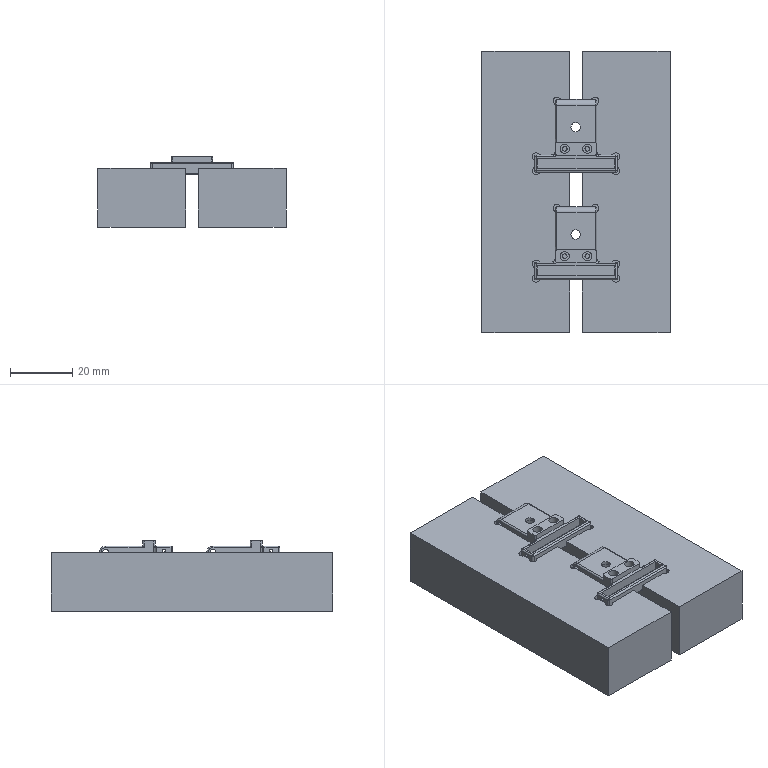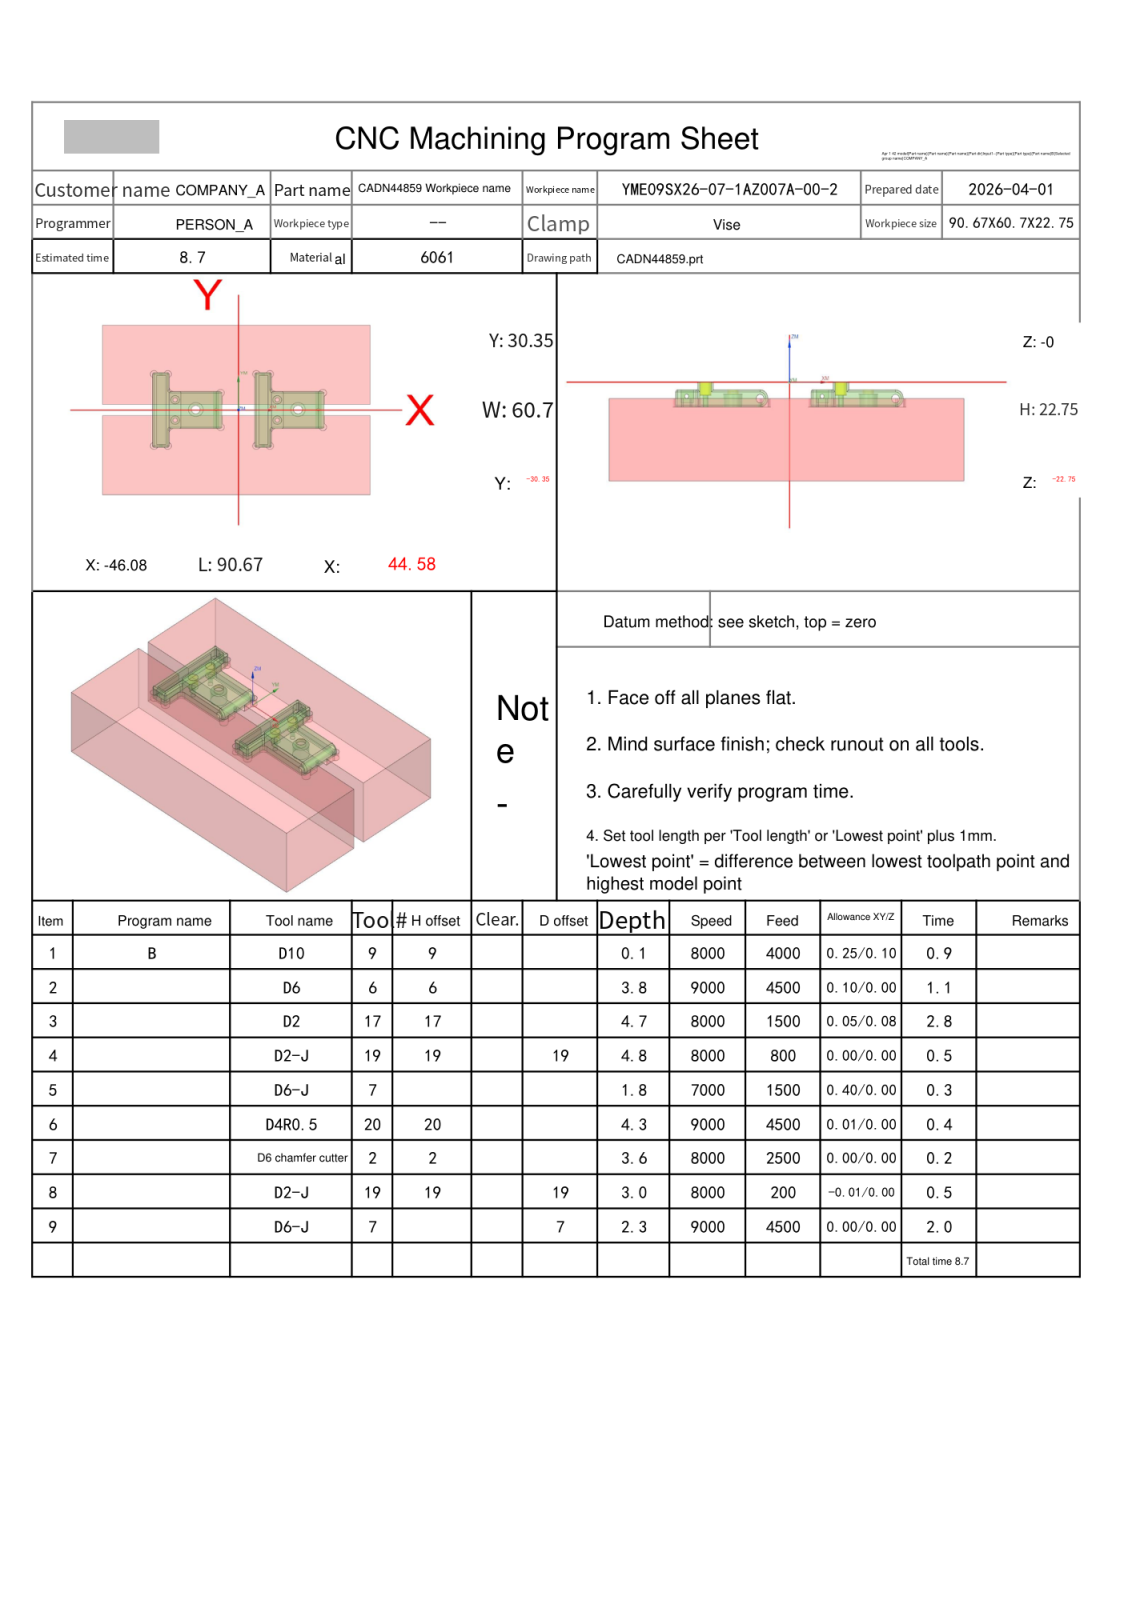NC program | NX | posted by the shop | part box 60.696 x 90.669 x 22.754 mm
Lines 1600 to 3624 of 6042, first 1509 of 2025 lines:
N3 T17 M06
(D2  D=2. R=0. H=17 ce=0.05 di=0.08)
G00 G90 G54 X-25.594 Y-2.915 M03 S8000
G43 H17 Z20.
M08
Z-.954
G01 Y11.298 Z-1.699 F1500.
X-26.646 Z-1.754
Y-11.298 Z-1.801
X-25.594 Z-1.803
Y11.298 Z-1.85
X-26.646 Z-1.852
Y-11.298 Z-1.899
X-25.594 Z-1.901
Y11.298 Z-1.948
X-26.646 Z-1.95
Y-11.298 Z-1.997
X-25.594 Z-1.999
Y11.298 Z-2.046
X-26.646 Z-2.048
Y-11.298 Z-2.095
X-25.594 Z-2.097
Y11.298 Z-2.144
X-26.646 Z-2.146
Y-11.298 Z-2.193
X-25.594 Z-2.195
Y11.298 Z-2.242
X-26.646 Z-2.244
Y-11.298 Z-2.291
X-25.594 Z-2.293
Y11.298 Z-2.34
X-26.646 Z-2.342
Y-11.298 Z-2.389
X-25.594 Z-2.391
Y11.298 Z-2.438
X-26.646 Z-2.44
Y-11.298 Z-2.487
X-25.594 Z-2.489
Y11.298 Z-2.536
X-26.646 Z-2.538
Y-11.298 Z-2.585
X-25.594 Z-2.587
Y11.298 Z-2.634
X-26.646 Z-2.636
Y-11.298 Z-2.683
X-25.594 Z-2.685
Y11.298 Z-2.732
X-26.646 Z-2.734
Y-11.298 Z-2.781
X-25.594 Z-2.783
Y11.298 Z-2.83
X-26.646 Z-2.832
Y-11.298 Z-2.879
X-25.594 Z-2.881
Y11.298 Z-2.928
X-26.646 Z-2.93
Y-11.298 Z-2.977
X-25.594 Z-2.979
Y11.298 Z-3.026
X-26.646 Z-3.028
Y-11.298 Z-3.075
X-25.594 Z-3.077
Y11.298 Z-3.124
X-26.646 Z-3.126
Y-11.298 Z-3.173
X-25.594 Z-3.175
Y11.298 Z-3.222
X-26.646 Z-3.224
Y-11.298 Z-3.271
X-25.594 Z-3.273
Y11.298 Z-3.32
X-26.646 Z-3.322
Y-11.298 Z-3.369
X-25.594 Z-3.371
Y11.298 Z-3.418
X-26.646 Z-3.42
Y-11.298 Z-3.467
X-25.594 Z-3.469
Y11.298 Z-3.516
X-26.646 Z-3.518
Y-11.298 Z-3.565
X-25.594 Z-3.567
Y11.298 Z-3.614
X-26.646 Z-3.616
Y-11.298 Z-3.663
X-25.594 Z-3.665
Y11.298 Z-3.712
X-26.646 Z-3.714
Y-11.298 Z-3.761
X-25.594 Z-3.763
Y11.298 Z-3.81
X-26.646 Z-3.812
Y-11.298 Z-3.859
X-25.594 Z-3.861
Y11.298 Z-3.908
X-26.646 Z-3.91
Y-11.298 Z-3.957
X-25.594 Z-3.959
Y11.298 Z-4.006
X-26.646 Z-4.008
Y-11.298 Z-4.055
X-25.594 Z-4.057
Y11.298 Z-4.104
X-26.646 Z-4.106
Y-11.298 Z-4.153
X-25.594 Z-4.155
Y11.298 Z-4.202
X-26.646 Z-4.204
Y-11.298 Z-4.251
X-25.594 Z-4.253
Y11.298 Z-4.3
X-26.646 Z-4.302
Y-11.298 Z-4.349
X-25.594 Z-4.351
Y11.298 Z-4.398
X-26.646 Z-4.4
Y-11.298 Z-4.447
X-25.594 Z-4.449
Y11.298 Z-4.496
X-26.646 Z-4.498
Y-11.298 Z-4.545
X-25.594 Z-4.547
Y11.298 Z-4.594
X-26.646 Z-4.596
Y-11.298 Z-4.643
X-25.594 Z-4.645
Y11.298 Z-4.692
X-26.646 Z-4.694
Y-11.298
X-25.594
Y11.298
X-26.646
Y10.898
Z-3.894
G00 Z20.
X9.006 Y-2.915
Z-.954
G01 Y11.298 Z-1.699
X7.954 Z-1.754
Y-11.298 Z-1.801
X9.006 Z-1.803
Y11.298 Z-1.85
X7.954 Z-1.852
Y-11.298 Z-1.899
X9.006 Z-1.901
Y11.298 Z-1.948
X7.954 Z-1.95
Y-11.298 Z-1.997
X9.006 Z-1.999
Y11.298 Z-2.046
X7.954 Z-2.048
Y-11.298 Z-2.095
X9.006 Z-2.097
Y11.298 Z-2.144
X7.954 Z-2.146
Y-11.298 Z-2.193
X9.006 Z-2.195
Y11.298 Z-2.242
X7.954 Z-2.244
Y-11.298 Z-2.291
X9.006 Z-2.293
Y11.298 Z-2.34
X7.954 Z-2.342
Y-11.298 Z-2.389
X9.006 Z-2.391
Y11.298 Z-2.438
X7.954 Z-2.44
Y-11.298 Z-2.487
X9.006 Z-2.489
Y11.298 Z-2.536
X7.954 Z-2.538
Y-11.298 Z-2.585
X9.006 Z-2.587
Y11.298 Z-2.634
X7.954 Z-2.636
Y-11.298 Z-2.683
X9.006 Z-2.685
Y11.298 Z-2.732
X7.954 Z-2.734
Y-11.298 Z-2.781
X9.006 Z-2.783
Y11.298 Z-2.83
X7.954 Z-2.832
Y-11.298 Z-2.879
X9.006 Z-2.881
Y11.298 Z-2.928
X7.954 Z-2.93
Y-11.298 Z-2.977
X9.006 Z-2.979
Y11.298 Z-3.026
X7.954 Z-3.028
Y-11.298 Z-3.075
X9.006 Z-3.077
Y11.298 Z-3.124
X7.954 Z-3.126
Y-11.298 Z-3.173
X9.006 Z-3.175
Y11.298 Z-3.222
X7.954 Z-3.224
Y-11.298 Z-3.271
X9.006 Z-3.273
Y11.298 Z-3.32
X7.954 Z-3.322
Y-11.298 Z-3.369
X9.006 Z-3.371
Y11.298 Z-3.418
X7.954 Z-3.42
Y-11.298 Z-3.467
X9.006 Z-3.469
Y11.298 Z-3.516
X7.954 Z-3.518
Y-11.298 Z-3.565
X9.006 Z-3.567
Y11.298 Z-3.614
X7.954 Z-3.616
Y-11.298 Z-3.663
X9.006 Z-3.665
Y11.298 Z-3.712
X7.954 Z-3.714
Y-11.298 Z-3.761
X9.006 Z-3.763
Y11.298 Z-3.81
X7.954 Z-3.812
Y-11.298 Z-3.859
X9.006 Z-3.861
Y11.298 Z-3.908
X7.954 Z-3.91
Y-11.298 Z-3.957
X9.006 Z-3.959
Y11.298 Z-4.006
X7.954 Z-4.008
Y-11.298 Z-4.055
X9.006 Z-4.057
Y11.298 Z-4.104
X7.954 Z-4.106
Y-11.298 Z-4.153
X9.006 Z-4.155
Y11.298 Z-4.202
X7.954 Z-4.204
Y-11.298 Z-4.251
X9.006 Z-4.253
Y11.298 Z-4.3
X7.954 Z-4.302
Y-11.298 Z-4.349
X9.006 Z-4.351
Y11.298 Z-4.398
X7.954 Z-4.4
Y-11.298 Z-4.447
X9.006 Z-4.449
Y11.298 Z-4.496
X7.954 Z-4.498
Y-11.298 Z-4.545
X9.006 Z-4.547
Y11.298 Z-4.594
X7.954 Z-4.596
Y-11.298 Z-4.643
X9.006 Z-4.645
Y11.298 Z-4.692
X7.954 Z-4.694
Y-11.298
X9.006
Y11.298
X7.954
Y10.898
Z-3.894
G00 Z20.
G00 G90 X13.59 Y3.809 M03 S8000
Z20.
Z.8
G01 X13.315 Y4.084 Z.78 F500.
X12.981 Z.762
X12.698 Y3.801 Z.741
Y3.471 Z.724
X12.981 Y3.184 Z.702
X13.315 Z.685
X13.598 Y3.467 Z.664
Y3.801 Z.646
X13.315 Y4.084 Z.625
X12.981 Z.608
X12.698 Y3.801 Z.587
Y3.471 Z.57
X12.981 Y3.184 Z.548
X13.315 Z.531
X13.598 Y3.467 Z.51
Y3.801 Z.492
X13.315 Y4.084 Z.471
X12.981 Z.454
X12.698 Y3.801 Z.433
Y3.471 Z.416
X12.981 Y3.184 Z.394
X13.315 Z.377
X13.598 Y3.467 Z.356
Y3.801 Z.338
X13.315 Y4.084 Z.317
X12.981 Z.3
X12.698 Y3.801 Z.279
Y3.471 Z.261
X12.981 Y3.184 Z.24
X13.315 Z.222
X13.598 Y3.467 Z.201
Y3.801 Z.184
X13.315 Y4.084 Z.163
X12.981 Z.145
X12.698 Y3.801 Z.124
Y3.471 Z.107
X12.981 Y3.184 Z.086
X13.315 Z.068
X13.598 Y3.467 Z.047
Y3.801 Z.03
X13.315 Y4.084 Z.009
X13.148 Z0.0
G03 X12.698 Y3.634 Z-.025 I0.0 J-.45
X12.802 Y3.346 Z-.035 I.45 J0.0
X13.148 Y3.184 Z-.049 I.346 J.288
X13.598 Y3.634 Z-.074 I0.0 J.45
X13.148 Y4.084 Z-.098 I-.45 J0.0
X12.698 Y3.634 Z-.123 I0.0 J-.45
X12.802 Y3.346 Z-.133 I.45 J0.0
X13.148 Y3.184 Z-.147 I.346 J.288
X13.598 Y3.634 Z-.172 I0.0 J.45
X13.148 Y4.084 Z-.196 I-.45 J0.0
X12.698 Y3.634 Z-.22 I0.0 J-.45
X12.802 Y3.346 Z-.231 I.45 J0.0
X13.148 Y3.184 Z-.245 I.346 J.288
X13.598 Y3.634 Z-.269 I0.0 J.45
X13.148 Y4.084 Z-.294 I-.45 J0.0
X12.698 Y3.634 Z-.318 I0.0 J-.45
X12.802 Y3.346 Z-.329 I.45 J0.0
X13.148 Y3.184 Z-.343 I.346 J.288
X13.598 Y3.634 Z-.367 I0.0 J.45
X13.148 Y4.084 Z-.392 I-.45 J0.0
X12.698 Y3.634 Z-.416 I0.0 J-.45
X12.802 Y3.346 Z-.427 I.45 J0.0
X13.148 Y3.184 Z-.441 I.346 J.288
X13.598 Y3.634 Z-.465 I0.0 J.45
X13.148 Y4.084 Z-.49 I-.45 J0.0
X12.698 Y3.634 Z-.514 I0.0 J-.45
X12.802 Y3.346 Z-.525 I.45 J0.0
X13.148 Y3.184 Z-.539 I.346 J.288
X13.598 Y3.634 Z-.563 I0.0 J.45
X13.148 Y4.084 Z-.588 I-.45 J0.0
X12.698 Y3.634 Z-.612 I0.0 J-.45
X12.802 Y3.346 Z-.623 I.45 J0.0
X13.148 Y3.184 Z-.637 I.346 J.288
X13.598 Y3.634 Z-.661 I0.0 J.45
X13.148 Y4.084 Z-.686 I-.45 J0.0
X12.698 Y3.634 Z-.71 I0.0 J-.45
X12.802 Y3.346 Z-.721 I.45 J0.0
X13.148 Y3.184 Z-.735 I.346 J.288
X13.598 Y3.634 Z-.759 I0.0 J.45
X13.148 Y4.084 Z-.784 I-.45 J0.0
X12.698 Y3.634 Z-.808 I0.0 J-.45
X12.802 Y3.346 Z-.819 I.45 J0.0
X13.148 Y3.184 Z-.833 I.346 J.288
X13.598 Y3.634 Z-.857 I0.0 J.45
X13.148 Y4.084 Z-.882 I-.45 J0.0
X12.698 Y3.634 Z-.906 I0.0 J-.45
X12.802 Y3.346 Z-.917 I.45 J0.0
X13.148 Y3.184 Z-.931 I.346 J.288
X13.598 Y3.634 Z-.955 I0.0 J.45
X13.148 Y4.084 Z-.98 I-.45 J0.0
X12.698 Y3.634 Z-1.004 I0.0 J-.45
X12.802 Y3.346 Z-1.015 I.45 J0.0
X13.148 Y3.184 Z-1.029 I.346 J.288
X13.598 Y3.634 Z-1.053 I0.0 J.45
X13.148 Y4.084 Z-1.078 I-.45 J0.0
X12.698 Y3.634 Z-1.102 I0.0 J-.45
X12.802 Y3.346 Z-1.113 I.45 J0.0
X13.148 Y3.184 Z-1.127 I.346 J.288
X13.598 Y3.634 Z-1.151 I0.0 J.45
X13.148 Y4.084 Z-1.176 I-.45 J0.0
X12.698 Y3.634 Z-1.2 I0.0 J-.45
X12.802 Y3.346 Z-1.211 I.45 J0.0
X13.148 Y3.184 Z-1.225 I.346 J.288
X13.598 Y3.634 Z-1.249 I0.0 J.45
X13.148 Y4.084 Z-1.274 I-.45 J0.0
X12.698 Y3.634 Z-1.298 I0.0 J-.45
X12.802 Y3.346 Z-1.309 I.45 J0.0
X13.148 Y3.184 Z-1.323 I.346 J.288
X13.598 Y3.634 Z-1.347 I0.0 J.45
X13.148 Y4.084 Z-1.372 I-.45 J0.0
X12.698 Y3.634 Z-1.396 I0.0 J-.45
X12.802 Y3.346 Z-1.407 I.45 J0.0
X13.148 Y3.184 Z-1.421 I.346 J.288
X13.598 Y3.634 Z-1.445 I0.0 J.45
X13.148 Y4.084 Z-1.47 I-.45 J0.0
X12.698 Y3.634 Z-1.494 I0.0 J-.45
X12.802 Y3.346 Z-1.505 I.45 J0.0
X13.148 Y3.184 Z-1.519 I.346 J.288
X13.598 Y3.634 Z-1.543 I0.0 J.45
X13.148 Y4.084 Z-1.568 I-.45 J0.0
X12.698 Y3.634 Z-1.592 I0.0 J-.45
X12.802 Y3.346 Z-1.603 I.45 J0.0
X13.148 Y3.184 Z-1.617 I.346 J.288
X13.598 Y3.634 Z-1.641 I0.0 J.45
X13.148 Y4.084 Z-1.666 I-.45 J0.0
X12.698 Y3.634 Z-1.69 I0.0 J-.45
X12.802 Y3.346 Z-1.701 I.45 J0.0
X13.148 Y3.184 Z-1.715 I.346 J.288
X13.598 Y3.634 Z-1.739 I0.0 J.45
X13.148 Y4.084 Z-1.764 I-.45 J0.0
X12.698 Y3.634 Z-1.788 I0.0 J-.45
X12.802 Y3.346 Z-1.799 I.45 J0.0
X13.148 Y3.184 Z-1.813 I.346 J.288
X13.598 Y3.634 Z-1.837 I0.0 J.45
X13.148 Y4.084 Z-1.862 I-.45 J0.0
X12.698 Y3.634 Z-1.886 I0.0 J-.45
X12.802 Y3.346 Z-1.897 I.45 J0.0
X13.148 Y3.184 Z-1.911 I.346 J.288
X13.598 Y3.634 Z-1.935 I0.0 J.45
X13.148 Y4.084 Z-1.96 I-.45 J0.0
X12.698 Y3.634 Z-1.984 I0.0 J-.45
X12.802 Y3.346 Z-1.995 I.45 J0.0
X13.148 Y3.184 Z-2.009 I.346 J.288
X13.598 Y3.634 Z-2.033 I0.0 J.45
X13.148 Y4.084 Z-2.058 I-.45 J0.0
X12.698 Y3.634 Z-2.082 I0.0 J-.45
X12.802 Y3.346 Z-2.093 I.45 J0.0
X13.148 Y3.184 Z-2.107 I.346 J.288
X13.598 Y3.634 Z-2.131 I0.0 J.45
X13.148 Y4.084 Z-2.156 I-.45 J0.0
X12.698 Y3.634 Z-2.18 I0.0 J-.45
X12.802 Y3.346 Z-2.191 I.45 J0.0
X13.148 Y3.184 Z-2.205 I.346 J.288
X13.598 Y3.634 Z-2.229 I0.0 J.45
X13.148 Y4.084 Z-2.254 I-.45 J0.0
X12.698 Y3.634 Z-2.278 I0.0 J-.45
X12.802 Y3.346 Z-2.289 I.45 J0.0
X13.148 Y3.184 Z-2.303 I.346 J.288
X13.598 Y3.634 Z-2.327 I0.0 J.45
X13.148 Y4.084 Z-2.352 I-.45 J0.0
X12.698 Y3.634 Z-2.376 I0.0 J-.45
X12.802 Y3.346 Z-2.387 I.45 J0.0
X13.148 Y3.184 Z-2.401 I.346 J.288
X13.598 Y3.634 Z-2.425 I0.0 J.45
X13.148 Y4.084 Z-2.45 I-.45 J0.0
X12.698 Y3.634 Z-2.474 I0.0 J-.45
X12.802 Y3.346 Z-2.485 I.45 J0.0
X13.148 Y3.184 Z-2.499 I.346 J.288
X13.598 Y3.634 Z-2.523 I0.0 J.45
X13.148 Y4.084 Z-2.548 I-.45 J0.0
X12.698 Y3.634 Z-2.572 I0.0 J-.45
X12.802 Y3.346 Z-2.583 I.45 J0.0
X13.148 Y3.184 Z-2.597 I.346 J.288
X13.598 Y3.634 Z-2.621 I0.0 J.45
X13.148 Y4.084 Z-2.646 I-.45 J0.0
X12.698 Y3.634 Z-2.67 I0.0 J-.45
X12.802 Y3.346 Z-2.681 I.45 J0.0
X13.148 Y3.184 Z-2.695 I.346 J.288
X13.598 Y3.634 Z-2.719 I0.0 J.45
X13.148 Y4.084 Z-2.744 I-.45 J0.0
X12.698 Y3.634 Z-2.768 I0.0 J-.45
X12.802 Y3.346 Z-2.779 I.45 J0.0
X13.148 Y3.184 Z-2.793 I.346 J.288
X13.598 Y3.634 Z-2.817 I0.0 J.45
X13.148 Y4.084 Z-2.842 I-.45 J0.0
X12.698 Y3.634 Z-2.866 I0.0 J-.45
X12.802 Y3.346 Z-2.877 I.45 J0.0
X13.148 Y3.184 Z-2.891 I.346 J.288
X13.598 Y3.634 Z-2.915 I0.0 J.45
X13.148 Y4.084 Z-2.94 I-.45 J0.0
X12.698 Y3.634 I0.0 J-.45
X13.148 Y3.184 I.45 J0.0
X13.598 Y3.634 I0.0 J.45
X13.148 Y4.084 I-.45 J0.0
X12.798 Y3.917 I0.0 J-.45
G01 Z-2.14
G00 Z20.
X12.698 Y-3.788
Z.8
G01 Y-3.801 Z.799
X12.981 Y-4.084 Z.778
X13.315 Z.761
X13.598 Y-3.801 Z.74
Y-3.467 Z.722
X13.315 Y-3.184 Z.701
X12.981 Z.684
X12.698 Y-3.467 Z.663
Y-3.801 Z.645
X12.981 Y-4.084 Z.624
X13.315 Z.607
X13.598 Y-3.801 Z.586
Y-3.467 Z.568
X13.315 Y-3.184 Z.547
X12.981 Z.53
X12.698 Y-3.467 Z.509
Y-3.801 Z.491
X12.981 Y-4.084 Z.471
X13.315 Z.453
X13.598 Y-3.801 Z.432
Y-3.467 Z.415
X13.315 Y-3.184 Z.394
X12.981 Z.376
X12.698 Y-3.467 Z.355
Y-3.801 Z.338
X12.981 Y-4.084 Z.317
X13.315 Z.299
X13.598 Y-3.801 Z.278
Y-3.467 Z.261
X13.315 Y-3.184 Z.24
X12.981 Z.222
X12.698 Y-3.467 Z.201
Y-3.801 Z.184
X12.981 Y-4.084 Z.163
X13.315 Z.145
X13.598 Y-3.801 Z.124
Y-3.467 Z.107
X13.315 Y-3.184 Z.086
X12.981 Z.068
X12.698 Y-3.467 Z.047
Y-3.801 Z.03
X12.981 Y-4.084 Z.009
X13.148 Z0.0
G03 X13.598 Y-3.634 Z-.025 I0.0 J.45
X13.148 Y-3.184 Z-.049 I-.45 J0.0
X12.698 Y-3.634 Z-.074 I0.0 J-.45
X13.148 Y-4.084 Z-.098 I.45 J0.0
X13.598 Y-3.634 Z-.123 I0.0 J.45
X13.148 Y-3.184 Z-.147 I-.45 J0.0
X12.698 Y-3.634 Z-.172 I0.0 J-.45
X13.148 Y-4.084 Z-.196 I.45 J0.0
X13.598 Y-3.634 Z-.22 I0.0 J.45
X13.148 Y-3.184 Z-.245 I-.45 J0.0
X12.698 Y-3.634 Z-.269 I0.0 J-.45
X13.148 Y-4.084 Z-.294 I.45 J0.0
X13.598 Y-3.634 Z-.318 I0.0 J.45
X13.148 Y-3.184 Z-.343 I-.45 J0.0
X12.698 Y-3.634 Z-.367 I0.0 J-.45
X13.148 Y-4.084 Z-.392 I.45 J0.0
X13.598 Y-3.634 Z-.416 I0.0 J.45
X13.148 Y-3.184 Z-.441 I-.45 J0.0
X12.698 Y-3.634 Z-.465 I0.0 J-.45
X13.148 Y-4.084 Z-.49 I.45 J0.0
X13.598 Y-3.634 Z-.514 I0.0 J.45
X13.148 Y-3.184 Z-.539 I-.45 J0.0
X12.698 Y-3.634 Z-.563 I0.0 J-.45
X13.148 Y-4.084 Z-.588 I.45 J0.0
X13.598 Y-3.634 Z-.612 I0.0 J.45
X13.148 Y-3.184 Z-.637 I-.45 J0.0
X12.698 Y-3.634 Z-.661 I0.0 J-.45
X13.148 Y-4.084 Z-.686 I.45 J0.0
X13.598 Y-3.634 Z-.71 I0.0 J.45
X13.148 Y-3.184 Z-.735 I-.45 J0.0
X12.698 Y-3.634 Z-.759 I0.0 J-.45
X13.148 Y-4.084 Z-.784 I.45 J0.0
X13.598 Y-3.634 Z-.808 I0.0 J.45
X13.148 Y-3.184 Z-.833 I-.45 J0.0
X12.698 Y-3.634 Z-.857 I0.0 J-.45
X13.148 Y-4.084 Z-.882 I.45 J0.0
X13.598 Y-3.634 Z-.906 I0.0 J.45
X13.148 Y-3.184 Z-.931 I-.45 J0.0
X12.698 Y-3.634 Z-.955 I0.0 J-.45
X13.148 Y-4.084 Z-.98 I.45 J0.0
X13.598 Y-3.634 Z-1.004 I0.0 J.45
X13.148 Y-3.184 Z-1.029 I-.45 J0.0
X12.698 Y-3.634 Z-1.053 I0.0 J-.45
X13.148 Y-4.084 Z-1.078 I.45 J0.0
X13.598 Y-3.634 Z-1.102 I0.0 J.45
X13.148 Y-3.184 Z-1.127 I-.45 J0.0
X12.698 Y-3.634 Z-1.151 I0.0 J-.45
X13.148 Y-4.084 Z-1.176 I.45 J0.0
X13.598 Y-3.634 Z-1.2 I0.0 J.45
X13.148 Y-3.184 Z-1.225 I-.45 J0.0
X12.698 Y-3.634 Z-1.249 I0.0 J-.45
X13.148 Y-4.084 Z-1.274 I.45 J0.0
X13.598 Y-3.634 Z-1.298 I0.0 J.45
X13.148 Y-3.184 Z-1.323 I-.45 J0.0
X12.698 Y-3.634 Z-1.347 I0.0 J-.45
X13.148 Y-4.084 Z-1.372 I.45 J0.0
X13.598 Y-3.634 Z-1.396 I0.0 J.45
X13.148 Y-3.184 Z-1.421 I-.45 J0.0
X12.698 Y-3.634 Z-1.445 I0.0 J-.45
X13.148 Y-4.084 Z-1.47 I.45 J0.0
X13.598 Y-3.634 Z-1.494 I0.0 J.45
X13.148 Y-3.184 Z-1.519 I-.45 J0.0
X12.698 Y-3.634 Z-1.543 I0.0 J-.45
X13.148 Y-4.084 Z-1.568 I.45 J0.0
X13.598 Y-3.634 Z-1.592 I0.0 J.45
X13.148 Y-3.184 Z-1.617 I-.45 J0.0
X12.698 Y-3.634 Z-1.641 I0.0 J-.45
X13.148 Y-4.084 Z-1.666 I.45 J0.0
X13.598 Y-3.634 Z-1.69 I0.0 J.45
X13.148 Y-3.184 Z-1.715 I-.45 J0.0
X12.698 Y-3.634 Z-1.739 I0.0 J-.45
X13.148 Y-4.084 Z-1.764 I.45 J0.0
X13.598 Y-3.634 Z-1.788 I0.0 J.45
X13.148 Y-3.184 Z-1.813 I-.45 J0.0
X12.698 Y-3.634 Z-1.837 I0.0 J-.45
X13.148 Y-4.084 Z-1.862 I.45 J0.0
X13.598 Y-3.634 Z-1.886 I0.0 J.45
X13.148 Y-3.184 Z-1.911 I-.45 J0.0
X12.698 Y-3.634 Z-1.935 I0.0 J-.45
X13.148 Y-4.084 Z-1.96 I.45 J0.0
X13.598 Y-3.634 Z-1.984 I0.0 J.45
X13.148 Y-3.184 Z-2.009 I-.45 J0.0
X12.698 Y-3.634 Z-2.033 I0.0 J-.45
X13.148 Y-4.084 Z-2.058 I.45 J0.0
X13.598 Y-3.634 Z-2.082 I0.0 J.45
X13.148 Y-3.184 Z-2.107 I-.45 J0.0
X12.698 Y-3.634 Z-2.131 I0.0 J-.45
X13.148 Y-4.084 Z-2.156 I.45 J0.0
X13.598 Y-3.634 Z-2.18 I0.0 J.45
X13.148 Y-3.184 Z-2.205 I-.45 J0.0
X12.698 Y-3.634 Z-2.229 I0.0 J-.45
X13.148 Y-4.084 Z-2.254 I.45 J0.0
X13.598 Y-3.634 Z-2.278 I0.0 J.45
X13.148 Y-3.184 Z-2.303 I-.45 J0.0
X12.698 Y-3.634 Z-2.327 I0.0 J-.45
X13.148 Y-4.084 Z-2.352 I.45 J0.0
X13.598 Y-3.634 Z-2.376 I0.0 J.45
X13.148 Y-3.184 Z-2.401 I-.45 J0.0
X12.698 Y-3.634 Z-2.425 I0.0 J-.45
X13.148 Y-4.084 Z-2.45 I.45 J0.0
X13.598 Y-3.634 Z-2.474 I0.0 J.45
X13.148 Y-3.184 Z-2.499 I-.45 J0.0
X12.698 Y-3.634 Z-2.523 I0.0 J-.45
X13.148 Y-4.084 Z-2.548 I.45 J0.0
X13.598 Y-3.634 Z-2.572 I0.0 J.45
X13.148 Y-3.184 Z-2.597 I-.45 J0.0
X12.698 Y-3.634 Z-2.621 I0.0 J-.45
X13.148 Y-4.084 Z-2.646 I.45 J0.0
X13.598 Y-3.634 Z-2.67 I0.0 J.45
X13.148 Y-3.184 Z-2.695 I-.45 J0.0
X12.698 Y-3.634 Z-2.719 I0.0 J-.45
X13.148 Y-4.084 Z-2.744 I.45 J0.0
X13.598 Y-3.634 Z-2.768 I0.0 J.45
X13.148 Y-3.184 Z-2.793 I-.45 J0.0
X12.698 Y-3.634 Z-2.817 I0.0 J-.45
X13.148 Y-4.084 Z-2.842 I.45 J0.0
X13.598 Y-3.634 Z-2.866 I0.0 J.45
X13.148 Y-3.184 Z-2.891 I-.45 J0.0
X12.698 Y-3.634 Z-2.915 I0.0 J-.45
X13.148 Y-4.084 Z-2.94 I.45 J0.0
X13.598 Y-3.634 I0.0 J.45
X13.148 Y-3.184 I-.45 J0.0
X12.698 Y-3.634 I0.0 J-.45
X13.148 Y-4.084 I.45 J0.0
X13.497 Y-3.917 I0.0 J.45
G01 Z-2.14
G00 Z20.
X-21.606 Y-3.184
Z.8
G01 X-21.619 Z.799
X-21.902 Y-3.467 Z.778
Y-3.801 Z.761
X-21.619 Y-4.084 Z.74
X-21.285 Z.722
X-21.002 Y-3.801 Z.701
Y-3.467 Z.684
X-21.285 Y-3.184 Z.663
X-21.619 Z.645
X-21.902 Y-3.467 Z.624
Y-3.801 Z.607
X-21.619 Y-4.084 Z.586
X-21.285 Z.568
X-21.002 Y-3.801 Z.547
Y-3.467 Z.53
X-21.285 Y-3.184 Z.509
X-21.619 Z.491
X-21.902 Y-3.467 Z.471
Y-3.801 Z.453
X-21.619 Y-4.084 Z.432
X-21.285 Z.415
X-21.002 Y-3.801 Z.394
Y-3.467 Z.376
X-21.285 Y-3.184 Z.355
X-21.619 Z.338
X-21.902 Y-3.467 Z.317
Y-3.801 Z.299
X-21.619 Y-4.084 Z.278
X-21.285 Z.261
X-21.002 Y-3.801 Z.24
Y-3.467 Z.222
X-21.285 Y-3.184 Z.201
X-21.619 Z.184
X-21.902 Y-3.467 Z.163
Y-3.801 Z.145
X-21.619 Y-4.084 Z.124
X-21.285 Z.107
X-21.002 Y-3.801 Z.086
Y-3.467 Z.068
X-21.285 Y-3.184 Z.047
X-21.619 Z.03
X-21.902 Y-3.467 Z.009
Y-3.634 Z0.0
G03 X-21.452 Y-4.084 Z-.025 I.45 J0.0
X-21.002 Y-3.634 Z-.049 I0.0 J.45
X-21.452 Y-3.184 Z-.074 I-.45 J0.0
X-21.902 Y-3.634 Z-.098 I0.0 J-.45
X-21.452 Y-4.084 Z-.123 I.45 J0.0
X-21.002 Y-3.634 Z-.147 I0.0 J.45
X-21.452 Y-3.184 Z-.172 I-.45 J0.0
X-21.902 Y-3.634 Z-.196 I0.0 J-.45
X-21.452 Y-4.084 Z-.22 I.45 J0.0
X-21.002 Y-3.634 Z-.245 I0.0 J.45
X-21.452 Y-3.184 Z-.269 I-.45 J0.0
X-21.902 Y-3.634 Z-.294 I0.0 J-.45
X-21.452 Y-4.084 Z-.318 I.45 J0.0
X-21.002 Y-3.634 Z-.343 I0.0 J.45
X-21.452 Y-3.184 Z-.367 I-.45 J0.0
X-21.902 Y-3.634 Z-.392 I0.0 J-.45
X-21.452 Y-4.084 Z-.416 I.45 J0.0
X-21.002 Y-3.634 Z-.441 I0.0 J.45
X-21.452 Y-3.184 Z-.465 I-.45 J0.0
X-21.902 Y-3.634 Z-.49 I0.0 J-.45
X-21.452 Y-4.084 Z-.514 I.45 J0.0
X-21.002 Y-3.634 Z-.539 I0.0 J.45
X-21.452 Y-3.184 Z-.563 I-.45 J0.0
X-21.902 Y-3.634 Z-.588 I0.0 J-.45
X-21.452 Y-4.084 Z-.612 I.45 J0.0
X-21.002 Y-3.634 Z-.637 I0.0 J.45
X-21.452 Y-3.184 Z-.661 I-.45 J0.0
X-21.902 Y-3.634 Z-.686 I0.0 J-.45
X-21.452 Y-4.084 Z-.71 I.45 J0.0
X-21.002 Y-3.634 Z-.735 I0.0 J.45
X-21.452 Y-3.184 Z-.759 I-.45 J0.0
X-21.902 Y-3.634 Z-.784 I0.0 J-.45
X-21.452 Y-4.084 Z-.808 I.45 J0.0
X-21.002 Y-3.634 Z-.833 I0.0 J.45
X-21.452 Y-3.184 Z-.857 I-.45 J0.0
X-21.902 Y-3.634 Z-.882 I0.0 J-.45
X-21.452 Y-4.084 Z-.906 I.45 J0.0
X-21.002 Y-3.634 Z-.931 I0.0 J.45
X-21.452 Y-3.184 Z-.955 I-.45 J0.0
X-21.902 Y-3.634 Z-.98 I0.0 J-.45
X-21.452 Y-4.084 Z-1.004 I.45 J0.0
X-21.002 Y-3.634 Z-1.029 I0.0 J.45
X-21.452 Y-3.184 Z-1.053 I-.45 J0.0
X-21.902 Y-3.634 Z-1.078 I0.0 J-.45
X-21.452 Y-4.084 Z-1.102 I.45 J0.0
X-21.002 Y-3.634 Z-1.127 I0.0 J.45
X-21.452 Y-3.184 Z-1.151 I-.45 J0.0
X-21.902 Y-3.634 Z-1.176 I0.0 J-.45
X-21.452 Y-4.084 Z-1.2 I.45 J0.0
X-21.002 Y-3.634 Z-1.225 I0.0 J.45
X-21.452 Y-3.184 Z-1.249 I-.45 J0.0
X-21.902 Y-3.634 Z-1.274 I0.0 J-.45
X-21.452 Y-4.084 Z-1.298 I.45 J0.0
X-21.002 Y-3.634 Z-1.323 I0.0 J.45
X-21.452 Y-3.184 Z-1.347 I-.45 J0.0
X-21.902 Y-3.634 Z-1.372 I0.0 J-.45
X-21.452 Y-4.084 Z-1.396 I.45 J0.0
X-21.002 Y-3.634 Z-1.421 I0.0 J.45
X-21.452 Y-3.184 Z-1.445 I-.45 J0.0
X-21.902 Y-3.634 Z-1.47 I0.0 J-.45
X-21.452 Y-4.084 Z-1.494 I.45 J0.0
X-21.002 Y-3.634 Z-1.519 I0.0 J.45
X-21.452 Y-3.184 Z-1.543 I-.45 J0.0
X-21.902 Y-3.634 Z-1.568 I0.0 J-.45
X-21.452 Y-4.084 Z-1.592 I.45 J0.0
X-21.002 Y-3.634 Z-1.617 I0.0 J.45
X-21.452 Y-3.184 Z-1.641 I-.45 J0.0
X-21.902 Y-3.634 Z-1.666 I0.0 J-.45
X-21.452 Y-4.084 Z-1.69 I.45 J0.0
X-21.002 Y-3.634 Z-1.715 I0.0 J.45
X-21.452 Y-3.184 Z-1.739 I-.45 J0.0
X-21.902 Y-3.634 Z-1.764 I0.0 J-.45
X-21.452 Y-4.084 Z-1.788 I.45 J0.0
X-21.002 Y-3.634 Z-1.813 I0.0 J.45
X-21.452 Y-3.184 Z-1.837 I-.45 J0.0
X-21.902 Y-3.634 Z-1.862 I0.0 J-.45
X-21.452 Y-4.084 Z-1.886 I.45 J0.0
X-21.002 Y-3.634 Z-1.911 I0.0 J.45
X-21.452 Y-3.184 Z-1.935 I-.45 J0.0
X-21.902 Y-3.634 Z-1.96 I0.0 J-.45
X-21.452 Y-4.084 Z-1.984 I.45 J0.0
X-21.002 Y-3.634 Z-2.009 I0.0 J.45
X-21.452 Y-3.184 Z-2.033 I-.45 J0.0
X-21.902 Y-3.634 Z-2.058 I0.0 J-.45
X-21.452 Y-4.084 Z-2.082 I.45 J0.0
X-21.002 Y-3.634 Z-2.107 I0.0 J.45
X-21.452 Y-3.184 Z-2.131 I-.45 J0.0
X-21.902 Y-3.634 Z-2.156 I0.0 J-.45
X-21.452 Y-4.084 Z-2.18 I.45 J0.0
X-21.002 Y-3.634 Z-2.205 I0.0 J.45
X-21.452 Y-3.184 Z-2.229 I-.45 J0.0
X-21.902 Y-3.634 Z-2.254 I0.0 J-.45
X-21.452 Y-4.084 Z-2.278 I.45 J0.0
X-21.002 Y-3.634 Z-2.303 I0.0 J.45
X-21.452 Y-3.184 Z-2.327 I-.45 J0.0
X-21.902 Y-3.634 Z-2.352 I0.0 J-.45
X-21.452 Y-4.084 Z-2.376 I.45 J0.0
X-21.002 Y-3.634 Z-2.401 I0.0 J.45
X-21.452 Y-3.184 Z-2.425 I-.45 J0.0
X-21.902 Y-3.634 Z-2.45 I0.0 J-.45
X-21.452 Y-4.084 Z-2.474 I.45 J0.0
X-21.002 Y-3.634 Z-2.499 I0.0 J.45
X-21.452 Y-3.184 Z-2.523 I-.45 J0.0
X-21.902 Y-3.634 Z-2.548 I0.0 J-.45
X-21.452 Y-4.084 Z-2.572 I.45 J0.0
X-21.002 Y-3.634 Z-2.597 I0.0 J.45
X-21.452 Y-3.184 Z-2.621 I-.45 J0.0
X-21.902 Y-3.634 Z-2.646 I0.0 J-.45
X-21.452 Y-4.084 Z-2.67 I.45 J0.0
X-21.002 Y-3.634 Z-2.695 I0.0 J.45
X-21.452 Y-3.184 Z-2.719 I-.45 J0.0
X-21.902 Y-3.634 Z-2.744 I0.0 J-.45
X-21.452 Y-4.084 Z-2.768 I.45 J0.0
X-21.002 Y-3.634 Z-2.793 I0.0 J.45
X-21.452 Y-3.184 Z-2.817 I-.45 J0.0
X-21.902 Y-3.634 Z-2.842 I0.0 J-.45
X-21.452 Y-4.084 Z-2.866 I.45 J0.0
X-21.002 Y-3.634 Z-2.891 I0.0 J.45
X-21.452 Y-3.184 Z-2.915 I-.45 J0.0
X-21.902 Y-3.634 Z-2.94 I0.0 J-.45
X-21.452 Y-4.084 I.45 J0.0
X-21.002 Y-3.634 I0.0 J.45
X-21.452 Y-3.184 I-.45 J0.0
X-21.902 Y-3.634 I0.0 J-.45
X-21.736 Y-3.983 I.45 J0.0
G01 Z-2.14
G00 Z20.
X-21.606 Y4.084
Z.8
G01 X-21.619 Z.799
X-21.902 Y3.801 Z.778
Y3.467 Z.761
X-21.619 Y3.184 Z.74
X-21.285 Z.722
X-21.002 Y3.467 Z.701
Y3.801 Z.684
X-21.285 Y4.084 Z.663
X-21.619 Z.645
X-21.902 Y3.801 Z.624
Y3.467 Z.607
X-21.619 Y3.184 Z.586
X-21.285 Z.568
X-21.002 Y3.467 Z.547
Y3.801 Z.53
X-21.285 Y4.084 Z.509
X-21.619 Z.491
X-21.902 Y3.801 Z.471
Y3.467 Z.453
X-21.619 Y3.184 Z.432
X-21.285 Z.415
X-21.002 Y3.467 Z.394
Y3.801 Z.376
X-21.285 Y4.084 Z.355
X-21.619 Z.338
X-21.902 Y3.801 Z.317
Y3.467 Z.299
X-21.619 Y3.184 Z.278
X-21.285 Z.261
X-21.002 Y3.467 Z.24
Y3.801 Z.222
X-21.285 Y4.084 Z.201
X-21.619 Z.184
X-21.902 Y3.801 Z.163
Y3.467 Z.145
X-21.619 Y3.184 Z.124
X-21.285 Z.107
X-21.002 Y3.467 Z.086
Y3.801 Z.068
X-21.285 Y4.084 Z.047
X-21.619 Z.03
X-21.902 Y3.801 Z.009
Y3.634 Z0.0
G03 X-21.452 Y3.184 Z-.025 I.45 J0.0
X-21.002 Y3.634 Z-.049 I0.0 J.45
X-21.452 Y4.084 Z-.074 I-.45 J0.0
X-21.902 Y3.634 Z-.098 I0.0 J-.45
X-21.452 Y3.184 Z-.123 I.45 J0.0
X-21.002 Y3.634 Z-.147 I0.0 J.45
X-21.452 Y4.084 Z-.172 I-.45 J0.0
X-21.902 Y3.634 Z-.196 I0.0 J-.45
X-21.452 Y3.184 Z-.22 I.45 J0.0
X-21.002 Y3.634 Z-.245 I0.0 J.45
X-21.452 Y4.084 Z-.269 I-.45 J0.0
X-21.902 Y3.634 Z-.294 I0.0 J-.45
X-21.452 Y3.184 Z-.318 I.45 J0.0
X-21.002 Y3.634 Z-.343 I0.0 J.45
X-21.452 Y4.084 Z-.367 I-.45 J0.0
X-21.902 Y3.634 Z-.392 I0.0 J-.45
X-21.452 Y3.184 Z-.416 I.45 J0.0
X-21.002 Y3.634 Z-.441 I0.0 J.45
X-21.452 Y4.084 Z-.465 I-.45 J0.0
X-21.902 Y3.634 Z-.49 I0.0 J-.45
X-21.452 Y3.184 Z-.514 I.45 J0.0
X-21.002 Y3.634 Z-.539 I0.0 J.45
X-21.452 Y4.084 Z-.563 I-.45 J0.0
X-21.902 Y3.634 Z-.588 I0.0 J-.45
X-21.452 Y3.184 Z-.612 I.45 J0.0
X-21.002 Y3.634 Z-.637 I0.0 J.45
X-21.452 Y4.084 Z-.661 I-.45 J0.0
X-21.902 Y3.634 Z-.686 I0.0 J-.45
X-21.452 Y3.184 Z-.71 I.45 J0.0
X-21.002 Y3.634 Z-.735 I0.0 J.45
X-21.452 Y4.084 Z-.759 I-.45 J0.0
X-21.902 Y3.634 Z-.784 I0.0 J-.45
X-21.452 Y3.184 Z-.808 I.45 J0.0
X-21.002 Y3.634 Z-.833 I0.0 J.45
X-21.452 Y4.084 Z-.857 I-.45 J0.0
X-21.902 Y3.634 Z-.882 I0.0 J-.45
X-21.452 Y3.184 Z-.906 I.45 J0.0
X-21.002 Y3.634 Z-.931 I0.0 J.45
X-21.452 Y4.084 Z-.955 I-.45 J0.0
X-21.902 Y3.634 Z-.98 I0.0 J-.45
X-21.452 Y3.184 Z-1.004 I.45 J0.0
X-21.002 Y3.634 Z-1.029 I0.0 J.45
X-21.452 Y4.084 Z-1.053 I-.45 J0.0
X-21.902 Y3.634 Z-1.078 I0.0 J-.45
X-21.452 Y3.184 Z-1.102 I.45 J0.0
X-21.002 Y3.634 Z-1.127 I0.0 J.45
X-21.452 Y4.084 Z-1.151 I-.45 J0.0
X-21.902 Y3.634 Z-1.176 I0.0 J-.45
X-21.452 Y3.184 Z-1.2 I.45 J0.0
X-21.002 Y3.634 Z-1.225 I0.0 J.45
X-21.452 Y4.084 Z-1.249 I-.45 J0.0
X-21.902 Y3.634 Z-1.274 I0.0 J-.45
X-21.452 Y3.184 Z-1.298 I.45 J0.0
X-21.002 Y3.634 Z-1.323 I0.0 J.45
X-21.452 Y4.084 Z-1.347 I-.45 J0.0
X-21.902 Y3.634 Z-1.372 I0.0 J-.45
X-21.452 Y3.184 Z-1.396 I.45 J0.0
X-21.002 Y3.634 Z-1.421 I0.0 J.45
X-21.452 Y4.084 Z-1.445 I-.45 J0.0
X-21.902 Y3.634 Z-1.47 I0.0 J-.45
X-21.452 Y3.184 Z-1.494 I.45 J0.0
X-21.002 Y3.634 Z-1.519 I0.0 J.45
X-21.452 Y4.084 Z-1.543 I-.45 J0.0
X-21.902 Y3.634 Z-1.568 I0.0 J-.45
X-21.452 Y3.184 Z-1.592 I.45 J0.0
X-21.002 Y3.634 Z-1.617 I0.0 J.45
X-21.452 Y4.084 Z-1.641 I-.45 J0.0
X-21.902 Y3.634 Z-1.666 I0.0 J-.45
X-21.452 Y3.184 Z-1.69 I.45 J0.0
X-21.002 Y3.634 Z-1.715 I0.0 J.45
X-21.452 Y4.084 Z-1.739 I-.45 J0.0
X-21.902 Y3.634 Z-1.764 I0.0 J-.45
X-21.452 Y3.184 Z-1.788 I.45 J0.0
X-21.002 Y3.634 Z-1.813 I0.0 J.45
X-21.452 Y4.084 Z-1.837 I-.45 J0.0
X-21.902 Y3.634 Z-1.862 I0.0 J-.45
X-21.452 Y3.184 Z-1.886 I.45 J0.0
X-21.002 Y3.634 Z-1.911 I0.0 J.45
X-21.452 Y4.084 Z-1.935 I-.45 J0.0
X-21.902 Y3.634 Z-1.96 I0.0 J-.45
X-21.452 Y3.184 Z-1.984 I.45 J0.0
X-21.002 Y3.634 Z-2.009 I0.0 J.45
X-21.452 Y4.084 Z-2.033 I-.45 J0.0
X-21.902 Y3.634 Z-2.058 I0.0 J-.45
X-21.452 Y3.184 Z-2.082 I.45 J0.0
X-21.002 Y3.634 Z-2.107 I0.0 J.45
X-21.452 Y4.084 Z-2.131 I-.45 J0.0
X-21.902 Y3.634 Z-2.156 I0.0 J-.45
X-21.452 Y3.184 Z-2.18 I.45 J0.0
X-21.002 Y3.634 Z-2.205 I0.0 J.45
X-21.452 Y4.084 Z-2.229 I-.45 J0.0
X-21.902 Y3.634 Z-2.254 I0.0 J-.45
X-21.452 Y3.184 Z-2.278 I.45 J0.0
X-21.002 Y3.634 Z-2.303 I0.0 J.45
X-21.452 Y4.084 Z-2.327 I-.45 J0.0
X-21.902 Y3.634 Z-2.352 I0.0 J-.45
X-21.452 Y3.184 Z-2.376 I.45 J0.0
X-21.002 Y3.634 Z-2.401 I0.0 J.45
X-21.452 Y4.084 Z-2.425 I-.45 J0.0
X-21.902 Y3.634 Z-2.45 I0.0 J-.45
X-21.452 Y3.184 Z-2.474 I.45 J0.0
X-21.002 Y3.634 Z-2.499 I0.0 J.45
X-21.452 Y4.084 Z-2.523 I-.45 J0.0
X-21.902 Y3.634 Z-2.548 I0.0 J-.45
X-21.452 Y3.184 Z-2.572 I.45 J0.0
X-21.002 Y3.634 Z-2.597 I0.0 J.45
X-21.452 Y4.084 Z-2.621 I-.45 J0.0
X-21.902 Y3.634 Z-2.646 I0.0 J-.45
X-21.452 Y3.184 Z-2.67 I.45 J0.0
X-21.002 Y3.634 Z-2.695 I0.0 J.45
X-21.452 Y4.084 Z-2.719 I-.45 J0.0
X-21.902 Y3.634 Z-2.744 I0.0 J-.45
X-21.452 Y3.184 Z-2.768 I.45 J0.0
X-21.002 Y3.634 Z-2.793 I0.0 J.45
X-21.452 Y4.084 Z-2.817 I-.45 J0.0
X-21.902 Y3.634 Z-2.842 I0.0 J-.45
X-21.452 Y3.184 Z-2.866 I.45 J0.0
X-21.002 Y3.634 Z-2.891 I0.0 J.45
X-21.452 Y4.084 Z-2.915 I-.45 J0.0
X-21.902 Y3.634 Z-2.94 I0.0 J-.45
X-21.452 Y3.184 I.45 J0.0
X-21.002 Y3.634 I0.0 J.45
X-21.452 Y4.084 I-.45 J0.0
X-21.902 Y3.634 I0.0 J-.45
X-21.736 Y3.284 I.45 J0.0
G01 Z-2.14
G00 Z20.
G91 G28 Z0.0
M05
M09
G91 G28 Z0.0
M01
N4 T19 M06
(D2-J  D=2. R=0. H=19 ce=0.00 di=0.00)
G00 G90 G54 X7.904 Y-2.909 M03 S8000
G43 H19 Z20.
M08
Z-1.254
G01 Y-11.348 Z-1.696 F800.
X9.006 Z-1.754
G41 D19
X9.056
Y11.348 Z-2.23
X7.904 Z-2.254
Y-11.348 Z-2.73
X9.056 Z-2.754
Y11.348 Z-3.23
X7.904 Z-3.254
Y-11.348 Z-3.73
X9.056 Z-3.754
Y11.348 Z-4.23
X7.904 Z-4.254
Y-11.348 Z-4.73
X9.056 Z-4.754
Y11.348
X7.904
Y-11.348
X9.056
Y-10.948
X9.053 Y-10.921
X9.033 Y-10.9
X9.006 Y-10.898
G40 X8.956
Z-3.754
G00 Z20.
X-25.544 Y2.909
Z-1.254
G01 Y11.348 Z-1.696
X-26.646 Z-1.754
G41 D19
X-26.696
Y-11.348 Z-2.23
X-25.544 Z-2.254
Y11.348 Z-2.73
X-26.696 Z-2.754
Y-11.348 Z-3.23
X-25.544 Z-3.254
Y11.348 Z-3.73
X-26.696 Z-3.754
Y-11.348 Z-4.23
X-25.544 Z-4.254
Y11.348 Z-4.73
X-26.696 Z-4.754
Y-11.348
X-25.544
Y11.348
X-26.696
Y10.948
X-26.694 Y10.921
X-26.674 Y10.9
X-26.646 Y10.898
G40 X-26.596
Z-3.754
G00 Z20.
G91 G28 Z0.0
M05
M09
G91 G28 Z0.0
M01
N5 T07 M06
(D6-J  D=6. R=0. H=00 ce=0.40 di=0.00)
G00 G90 G54 X-18.232 Y10.508 M03 S7000
G43 H00 Z11.95
M08
Z1.5
G01 Z0.0 F1500.
G03 X-18.852 Y9.457 I.579 J-1.051
G01 Y-8.991
G02 X-19.349 Y-9.581 I-.6 J0.0
X-19.952 Y-9.634 I-.604 J3.448
G01 X-20.452
G02 X-21.052 Y-9.034 I0.0 J.6
G01 Y9.634
G02 X-19.886 Y10.833 I1.2 J0.0
G01 Z1.5
G00 Z4.
X16.368 Y10.508
Z1.5
G01 Z0.0
G03 X15.748 Y9.457 I.579 J-1.051
G01 Y-8.991
G02 X15.251 Y-9.581 I-.6 J0.0
X14.648 Y-9.634 I-.604 J3.448
G01 X14.148
G02 X13.548 Y-9.034 I0.0 J.6
G01 Y9.634
G02 X14.714 Y10.833 I1.2 J0.0
G01 Z1.5
G00 Z11.95
G00 G90 X-32.784 Y-1.2 M03 S7000
Z11.95
Z-.254
G01 Z-1.754 F1500.
X-30.384
G03 X-29.184 Y0.0 I0.0 J1.2
G01 Y12.849
G02 X-28.586 Y13.448 I.6 J-.001
G01 X-23.951
G02 X-23.352 Y12.849 I-.001 J-.6
G01 Y12.381
X-21.209 Y10.238
X-21.174 Y10.154
X-21.294 Y10.034
X-22.952
G03 X-26.852 Y6.134 I0.0 J-3.9
G01 Y-6.134
G03 X-22.952 Y-10.034 I3.9 J0.0
G01 X-21.294
X-21.174 Y-10.154
X-21.209 Y-10.238
X-23.352 Y-12.381
Y-12.849
G02 X-23.952 Y-13.448 I-.6 J.001
G01 X-28.586
G02 X-29.184 Y-12.849 I.001 J.6
G01 Y0.0
Y1.
G03 X-30.384 Y2.2 I-1.2 J0.0
G01 X-32.784
Z-.254
G00 Z11.95
X-3.316 Y1.2
Z-.254
G01 Z-1.754
X-5.716
G03 X-6.916 Y0.0 I0.0 J-1.2
G01 Y-6.135
G02 X-7.514 Y-6.734 I-.6 J.001
G01 X-15.454
G02 X-16.052 Y-6.135 I.001 J.6
G01 Y6.135
G02 X-15.454 Y6.734 I.6 J-.001
G01 X-7.514
G02 X-6.916 Y6.135 I-.001 J-.6
G01 Y-3.
G02 X-7.516 Y-3.6 I-.6 J0.0
G01 X-7.632 Y-3.589
X-9.416 Y-3.234
X-9.533 Y-3.223
G03 X-10.024 Y-3.478 I0.0 J-.6
G02 X-10.514 Y-3.734 I-.491 J.344
G01 X-12.454
G02 X-13.052 Y-3.135 I.001 J.6
G01 Y3.135
G02 X-12.454 Y3.734 I.6 J-.001
G01 X-10.514
G02 X-9.916 Y3.135 I-.001 J-.6
G01 Y-3.
Y-3.135
G02 X-10.439 Y-3.729 I-.6 J.001
G03 X-11.487 Y-4.919 I.152 J-1.19
G01 X-11.477 Y-5.072
Y-10.334
Z-.254
G00 Z2.246
X1.816 Y-1.2
Z-.254
G01 Z-1.754
X4.216
G03 X5.416 Y0.0 I0.0 J1.2
G01 Y12.849
G02 X6.014 Y13.448 I.6 J-.001
G01 X10.649
G02 X11.248 Y12.849 I-.001 J-.6
G01 Y12.381
X13.391 Y10.238
X13.426 Y10.154
X13.306 Y10.034
X11.648
G03 X7.748 Y6.134 I0.0 J-3.9
G01 Y-6.134
G03 X11.648 Y-10.034 I3.9 J0.0
G01 X13.306
X13.426 Y-10.154
X13.391 Y-10.238
X11.248 Y-12.381
Y-12.849
G02 X10.648 Y-13.448 I-.6 J.001
G01 X6.014
G02 X5.416 Y-12.849 I.001 J.6
G01 Y0.0
Y1.
G03 X4.216 Y2.2 I-1.2 J0.0
G01 X1.816
Z-.254
G00 Z11.95
X31.284 Y1.2
Z-.254
G01 Z-1.754
X28.884
G03 X27.684 Y0.0 I0.0 J-1.2
G01 Y-6.135
G02 X27.086 Y-6.734 I-.6 J.001
G01 X19.146
G02 X18.548 Y-6.135 I.001 J.6
G01 Y6.135
G02 X19.146 Y6.734 I.6 J-.001
G01 X27.086
G02 X27.684 Y6.135 I-.001 J-.6
G01 Y-3.
G02 X27.084 Y-3.6 I-.6 J0.0
G01 X26.968 Y-3.589
X25.184 Y-3.234
X25.067 Y-3.223
G03 X24.576 Y-3.478 I0.0 J-.6
G02 X24.086 Y-3.734 I-.491 J.344
G01 X22.146
G02 X21.548 Y-3.135 I.001 J.6
G01 Y3.135
G02 X22.146 Y3.734 I.6 J-.001
G01 X24.086
G02 X24.684 Y3.135 I-.001 J-.6
G01 Y-3.
Y-3.135
G02 X24.161 Y-3.729 I-.6 J.001
G03 X23.113 Y-4.919 I.152 J-1.19
G01 X23.123 Y-5.072
Y-10.334
Z-.254
G00 Z11.95
G91 G28 Z0.0
M05
M09
G91 G28 Z0.0
M01
N6 T20 M06
(D4R0.5  D=4. R=0.5 H=20 ce=0.01 di=0.00)
G00 G90 G54 X24.306 Y9.777 M03 S9000
G43 H20 Z11.95
M08
Z-1.263
G01 Z-1.763 F4500.
Y9.749
G03 X25.972 Y7.777 I2. J0.0
G01 X25.986 Y7.775
X27.145 Y7.771
X27.28 Y7.752
G02 X28.806 Y6.134 I-.241 J-1.755
G01 Y-6.134
G02 X27.274 Y-7.753 I-1.774 J.144
G01 X27.145 Y-7.771
X25.986 Y-7.775
X25.972 Y-7.777
Y-7.817 Z-1.769
Y-7.849 Z-1.775
X27.138 Y-7.836
G03 X28.921 Y-6.134 I-.021 J1.808
G01 Y6.134
G03 X27.137 Y7.836 I-1.805 J-.107
G01 X25.972 Y7.849
Y7.885 Z-1.784
Y7.916 Z-1.792
X27.201 Y7.893
G02 X29.028 Y6.134 I-.035 J-1.864
G01 Y-6.134
G02 X27.201 Y-7.893 I-1.862 J.105
G01 X25.972 Y-7.916
Y-7.95 Z-1.802
Y-7.98 Z-1.812
X27.266 Y-7.954
G03 X29.131 Y-6.134 I-.038 J1.904
G01 Y6.134
G03 X27.267 Y7.954 I-1.903 J-.084
G01 X25.972 Y7.98
Y8.012 Z-1.824
Y8.042 Z-1.837
X27.347 Y8.016
X27.63 Y7.968
G02 X29.231 Y6.134 I-.371 J-1.94
G01 Y-6.134
G02 X27.63 Y-7.968 I-1.972 J.105
G01 X27.347 Y-8.016
X25.972 Y-8.042
Y-8.073 Z-1.851
Y-8.101 Z-1.865
X27.347 Y-8.078
X27.561 Y-8.048
G03 X29.33 Y-6.134 I-.285 J2.037
G01 Y6.134
G03 X27.56 Y8.048 I-2.053 J-.123
G01 X27.347 Y8.078
X25.972 Y8.101
Y8.131 Z-1.881
Y8.158 Z-1.897
G02 X26.51 Y8.18 I.537 J-6.78
X27.748 Y8.066 I0.0 J-6.802
X29.427 Y6.134 I-.374 J-2.02
G01 Y-6.134
G02 X27.748 Y-8.066 I-2.053 J.088
X26.51 Y-8.18 I-1.239 J6.685
X25.972 Y-8.158 I0.0 J6.798
G01 Y-8.187 Z-1.914
Y-8.214 Z-1.932
X27.347 Y-8.199
X27.63 Y-8.158
G03 X29.522 Y-6.134 I-.301 J2.176
G01 Y6.134
G03 X27.63 Y8.158 I-2.192 J-.152
G01 X27.347 Y8.199
X25.972 Y8.214
Y8.241 Z-1.952
Y8.267 Z-1.972
X27.347 Y8.248
X27.556 Y8.224
G02 X29.056 Y7.488 I-.281 J-2.472
X29.615 Y6.134 I-1.41 J-1.374
G01 Y-6.134
G02 X28.48 Y-7.929 I-2.114 J.08
X27.11 Y-8.261 I-1.37 J2.666
G01 X27.064 Y-8.26
X25.986
X25.972 Y-8.267
Y-8.293 Z-1.993
Y-8.317 Z-2.015
X27.244 Y-8.302
G03 X28.758 Y-7.836 I-.033 J2.799
X29.706 Y-6.134 I-1.174 J1.769
G01 Y6.135
G03 X29.364 Y7.225 I-1.904 J0.0
X27.63 Y8.266 I-2.03 J-1.417
G01 X27.347 Y8.301
X25.972 Y8.317
Y8.342 Z-2.038
Y8.365 Z-2.061
X27.347 Y8.351
X27.63 Y8.321
G02 X29.33 Y7.407 I-.307 J-2.608
X29.796 Y6.134 I-1.508 J-1.273
G01 Y-6.134
G02 X28.515 Y-8.053 I-2.208 J.086
X27.111 Y-8.361 I-1.404 J3.05
G01 X27.064 Y-8.36
X25.986
X25.972 Y-8.365
Y-8.388 Z-2.087
Y-8.41 Z-2.112
X27.347 Y-8.393
G03 X28.763 Y-7.985 I-.117 J3.068
X29.883 Y-6.134 I-1.087 J1.921
G01 Y6.134
G03 X29.33 Y7.531 I-2.243 J-.08
X27.63 Y8.365 I-1.999 J-1.922
G01 X27.347 Y8.393
X25.972 Y8.41
Y8.432 Z-2.138
Y8.452 Z-2.165
X27.347 Y8.437
X27.63 Y8.408
G02 X29.047 Y7.879 I-.298 J-2.954
X29.968 Y6.134 I-1.313 J-1.809
G01 Y-6.134
G02 X28.772 Y-8.053 I-2.254 J.072
X27.63 Y-8.408 I-1.466 J2.7
G01 X27.347 Y-8.437
X25.972 Y-8.452
Y-8.472 Z-2.194
X25.973 Y-8.491 Z-2.222
X27.347 Y-8.482
X27.63 Y-8.454
G03 X29.047 Y-7.953 I-.325 J3.171
X30.051 Y-6.134 I-1.243 J1.873
G01 Y6.134
G03 X29.047 Y7.953 I-2.247 J-.054
X27.63 Y8.454 I-1.741 J-2.67
G01 X27.347 Y8.482
X25.973 Y8.491
Y8.509 Z-2.252
Y8.526 Z-2.282
X27.347 Y8.515
X27.63 Y8.493
G02 X29.047 Y8.021 I-.292 J-3.234
X30.131 Y6.134 I-1.197 J-1.943
G01 Y-6.134
G02 X29.047 Y-8.021 I-2.281 J.056
X27.63 Y-8.493 I-1.708 J2.761
X26.494 Y-8.534 I-1.137 J15.796
X25.973 Y-8.526 I0.0 J15.837
G01 Y-8.542 Z-2.314
Y-8.557 Z-2.345
X27.347 Y-8.549
X27.63 Y-8.527
G03 X29.047 Y-8.085 I-.269 J3.352
X30.209 Y-6.134 I-1.147 J2.006
G01 Y6.134
G03 X29.047 Y8.085 I-2.31 J-.055
X27.63 Y8.527 I-1.685 J-2.91
G01 X27.347 Y8.549
X25.973 Y8.557
Y8.583 Z-2.412
X25.987 Y8.577
X27.347 Y8.572
X27.63 Y8.556
G02 X29.047 Y8.146 I-.231 J-3.446
X30.285 Y6.134 I-1.111 J-2.07
G01 Y-6.134
G02 X29.047 Y-8.146 I-2.349 J.058
X27.63 Y-8.556 I-1.647 J3.035
G01 X27.347 Y-8.572
X25.987 Y-8.577
X25.973 Y-8.583
Y-8.595 Z-2.446
Y-8.606 Z-2.481
G03 X26.445 Y-8.611 I.473 J21.519
X27.63 Y-8.578 I0.0 J21.525
X29.047 Y-8.205 I-.171 J3.516
X30.357 Y-6.134 I-1.073 J2.129
G01 Y6.134
G03 X29.047 Y8.205 I-2.383 J-.058
X27.63 Y8.578 I-1.587 J-3.142
G01 X27.347 Y8.595
X25.973 Y8.606
X25.984 Y8.623 Z-2.553
X27.369 Y8.618
X27.63 Y8.602
G02 X28.863 Y8.336 I-.168 J-3.769
X30.149 Y7.205 I-.926 J-2.35
X30.427 Y6.134 I-2.069 J-1.107
G01 Y-6.134
G02 X29.33 Y-8.089 I-2.368 J.043
X28.197 Y-8.534 I-1.688 J2.635
X27.121 Y-8.621 I-1.076 J6.583
G01 X27.064
X26.002
X25.984 Y-8.623
Y-8.636 Z-2.628
X26.002 Y-8.631
X27.274
G03 X28.219 Y-8.555 I0.0 J5.964
X29.33 Y-8.143 I-.482 J3.003
G01 X29.475 Y-8.053
G03 X30.493 Y-6.134 I-1.379 J1.962
G01 Y6.138
G03 X30.032 Y7.503 I-2.251 J0.0
X28.492 Y8.496 I-2.144 J-1.635
X27.301 Y8.631 I-1.19 J-5.183
G01 X26.002
X25.984 Y8.636
Y8.643 Z-2.705
G02 X26.46 Y8.646 I.476 J-38.285
X27.719 Y8.625 I0.0 J-38.288
X28.775 Y8.447 I-.132 J-3.998
X30.29 Y7.205 I-.773 J-2.488
X30.557 Y6.134 I-2.175 J-1.112
G01 Y-6.134
G02 X29.879 Y-7.771 I-2.394 J.033
X28.48 Y-8.528 I-1.968 J1.965
X27.908 Y-8.618 I-1.487 J7.543
X26.46 Y-8.646 I-1.448 J38.261
X25.984 Y-8.643 I0.0 J38.288
G01 X25.993 Y-8.644 Z-2.785
X26.214
X27.63 Y-8.638
X27.914 Y-8.625
G03 X29.628 Y-8.053 I-.085 J3.109
X30.618 Y-6.134 I-1.434 J1.954
G01 Y6.134
G03 X29.628 Y8.053 I-2.424 J-.035
X27.914 Y8.625 I-1.8 J-2.537
X26.679 Y8.652 I-1.234 J-28.793
X25.993 Y8.644 I0.0 J-28.819
G01 Z-2.867
X27.63
X28.02 Y8.629
G02 X29.613 Y8.116 I-.117 J-3.09
X30.675 Y6.134 I-1.393 J-2.022
G01 Y-6.134
G02 X29.613 Y-8.116 I-2.455 J.04
X28.021 Y-8.629 I-1.709 J2.576
G01 X27.63 Y-8.644
X25.993
Z-2.952
X27.63
X27.914 Y-8.641
X27.917
G03 X29.308 Y-8.336 I0.0 J3.323
X30.729 Y-6.134 I-1.06 J2.244
G01 Y6.134
G03 X29.308 Y8.336 I-2.481 J-.042
X27.916 Y8.641 I-1.392 J-3.019
G01 X27.914
X27.63 Y8.644
X25.993
Z-3.038
X27.914
X28.197 Y8.631
G02 X29.613 Y8.2 I-.097 J-2.861
X30.779 Y6.134 I-1.314 J-2.103
G01 Y-6.134
G02 X29.047 Y-8.472 I-2.517 J.054
X27.954 Y-8.644 I-1.092 J3.388
G01 X27.914
X25.993
Z-3.127
X27.914
X28.197 Y-8.637
G03 X29.435 Y-8.336 I-.063 J2.952
X30.826 Y-6.134 I-1.112 J2.242
G01 Y6.134
G03 X29.896 Y8.041 I-2.504 J-.04
X28.197 Y8.637 I-1.743 J-2.246
G01 X27.914 Y8.644
X25.993
Z-3.217
X28.197
G02 X29.33 Y8.409 I-.029 J-2.996
X30.869 Y6.134 I-.962 J-2.309
G01 Y-6.134
G02 X29.33 Y-8.409 I-2.501 J.034
X28.197 Y-8.644 I-1.162 J2.762
G01 X25.993
Z-3.309
X28.197